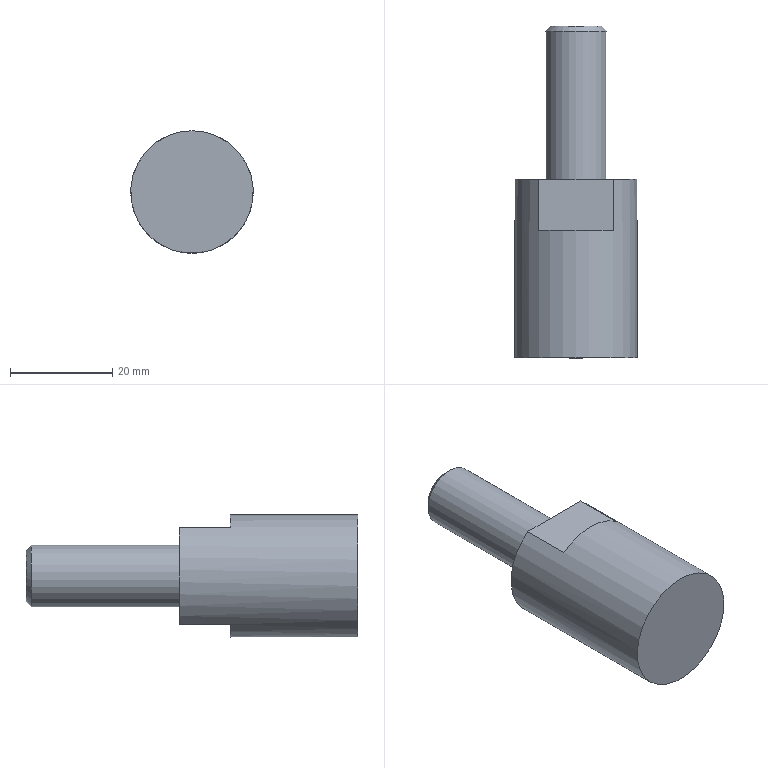Part | NX | features solid 2 | 1 solid | 10 faces | box 24 x 65 x 24 mm | volume 18709 mm3 | plane 7 | cylinder 2 | cone 1 | commonest cylinder face diameters 12 x1 24 x1
STEP:
#1=CARTESIAN_POINT('',(-265.,490.,-30.));
#2=VERTEX_POINT('',#1);
#3=CARTESIAN_POINT('',(-265.,490.,-25.));
#4=DIRECTION('',(0.,-1.,0.));
#5=DIRECTION('',(0.,0.,-1.));
#6=AXIS2_PLACEMENT_3D('',#3,#4,#5);
#7=CIRCLE('',#6,5.);
#8=EDGE_CURVE('',#2,#2,#7,.T.);
#9=ORIENTED_EDGE('',*,*,#8,.F.);
#10=EDGE_LOOP('',(#9));
#11=FACE_BOUND('',#10,.T.);
#12=CARTESIAN_POINT('',(-265.,490.,-25.));
#13=DIRECTION('',(0.,1.,0.));
#14=DIRECTION('',(0.,0.,-1.));
#15=AXIS2_PLACEMENT_3D('',#12,#13,#14);
#16=PLANE('',#15);
#17=ADVANCED_FACE('',(#11),#16,.T.);
#18=CARTESIAN_POINT('',(-265.,489.,-31.));
#19=VERTEX_POINT('',#18);
#20=CARTESIAN_POINT('',(-265.,489.,-25.));
#21=DIRECTION('',(0.,-1.,0.));
#22=DIRECTION('',(0.,0.,-1.));
#23=AXIS2_PLACEMENT_3D('',#20,#21,#22);
#24=CIRCLE('',#23,6.);
#25=EDGE_CURVE('',#19,#19,#24,.F.);
#26=ORIENTED_EDGE('',*,*,#25,.T.);
#27=EDGE_LOOP('',(#26));
#28=FACE_BOUND('',#27,.T.);
#29=ORIENTED_EDGE('',*,*,#8,.T.);
#30=EDGE_LOOP('',(#29));
#31=FACE_BOUND('',#30,.T.);
#32=CARTESIAN_POINT('',(-265.,490.,-25.));
#33=DIRECTION('',(0.,-1.,0.));
#34=DIRECTION('',(0.,0.,1.));
#35=AXIS2_PLACEMENT_3D('',#32,#33,#34);
#36=CONICAL_SURFACE('',#35,5.,0.7854);
#37=ADVANCED_FACE('',(#28,#31),#36,.T.);
#38=ORIENTED_EDGE('',*,*,#25,.F.);
#39=EDGE_LOOP('',(#38));
#40=FACE_BOUND('',#39,.T.);
#41=CARTESIAN_POINT('',(-265.,460.,-31.));
#42=VERTEX_POINT('',#41);
#43=CARTESIAN_POINT('',(-265.,460.,-25.));
#44=DIRECTION('',(0.,-1.,0.));
#45=DIRECTION('',(0.,0.,-1.));
#46=AXIS2_PLACEMENT_3D('',#43,#44,#45);
#47=CIRCLE('',#46,6.);
#48=EDGE_CURVE('',#42,#42,#47,.T.);
#49=ORIENTED_EDGE('',*,*,#48,.F.);
#50=EDGE_LOOP('',(#49));
#51=FACE_BOUND('',#50,.T.);
#52=CARTESIAN_POINT('',(-265.,460.,-25.));
#53=DIRECTION('',(0.,1.,0.));
#54=DIRECTION('',(0.,0.,-1.));
#55=AXIS2_PLACEMENT_3D('',#52,#53,#54);
#56=CYLINDRICAL_SURFACE('',#55,6.);
#57=ADVANCED_FACE('',(#40,#51),#56,.T.);
#58=CARTESIAN_POINT('',(-272.331,450.,-34.5));
#59=VERTEX_POINT('',#58);
#60=CARTESIAN_POINT('',(-257.669,450.,-34.5));
#61=VERTEX_POINT('',#60);
#62=CARTESIAN_POINT('',(-272.331,450.,-34.5));
#63=DIRECTION('',(1.,0.,0.));
#64=VECTOR('',#63,1000.);
#65=LINE('',#62,#64);
#66=EDGE_CURVE('',#59,#61,#65,.T.);
#67=ORIENTED_EDGE('',*,*,#66,.T.);
#68=CARTESIAN_POINT('',(-265.,450.,-25.));
#69=DIRECTION('',(0.,-1.,0.));
#70=DIRECTION('',(0.,0.,-1.));
#71=AXIS2_PLACEMENT_3D('',#68,#69,#70);
#72=CIRCLE('',#71,12.);
#73=EDGE_CURVE('',#59,#61,#72,.T.);
#74=ORIENTED_EDGE('',*,*,#73,.F.);
#75=EDGE_LOOP('',(#67,#74));
#76=FACE_BOUND('',#75,.T.);
#77=CARTESIAN_POINT('',(-272.331,450.,-25.));
#78=DIRECTION('',(0.,1.,0.));
#79=DIRECTION('',(0.,0.,-1.));
#80=AXIS2_PLACEMENT_3D('',#77,#78,#79);
#81=PLANE('',#80);
#82=ADVANCED_FACE('',(#76),#81,.T.);
#83=CARTESIAN_POINT('',(-257.669,450.,-15.5));
#84=VERTEX_POINT('',#83);
#85=CARTESIAN_POINT('',(-272.331,450.,-15.5));
#86=VERTEX_POINT('',#85);
#87=CARTESIAN_POINT('',(-265.,450.,-25.));
#88=DIRECTION('',(0.,-1.,0.));
#89=DIRECTION('',(0.,0.,-1.));
#90=AXIS2_PLACEMENT_3D('',#87,#88,#89);
#91=CIRCLE('',#90,12.);
#92=EDGE_CURVE('',#84,#86,#91,.T.);
#93=ORIENTED_EDGE('',*,*,#92,.F.);
#94=CARTESIAN_POINT('',(-272.331,450.,-15.5));
#95=DIRECTION('',(1.,0.,0.));
#96=VECTOR('',#95,1000.);
#97=LINE('',#94,#96);
#98=EDGE_CURVE('',#86,#84,#97,.T.);
#99=ORIENTED_EDGE('',*,*,#98,.F.);
#100=EDGE_LOOP('',(#93,#99));
#101=FACE_BOUND('',#100,.T.);
#102=CARTESIAN_POINT('',(-268.666,450.,-26.25));
#103=DIRECTION('',(0.,1.,0.));
#104=DIRECTION('',(0.,0.,-1.));
#105=AXIS2_PLACEMENT_3D('',#102,#103,#104);
#106=PLANE('',#105);
#107=ADVANCED_FACE('',(#101),#106,.T.);
#108=CARTESIAN_POINT('',(-272.331,460.,-15.5));
#109=VERTEX_POINT('',#108);
#110=CARTESIAN_POINT('',(-257.669,460.,-15.5));
#111=VERTEX_POINT('',#110);
#112=CARTESIAN_POINT('',(-272.331,460.,-15.5));
#113=DIRECTION('',(1.,0.,0.));
#114=VECTOR('',#113,1000.);
#115=LINE('',#112,#114);
#116=EDGE_CURVE('',#109,#111,#115,.T.);
#117=ORIENTED_EDGE('',*,*,#116,.F.);
#118=CARTESIAN_POINT('',(-272.331,450.,-15.5));
#119=DIRECTION('',(0.,1.,0.));
#120=VECTOR('',#119,1000.);
#121=LINE('',#118,#120);
#122=EDGE_CURVE('',#109,#86,#121,.F.);
#123=ORIENTED_EDGE('',*,*,#122,.T.);
#124=ORIENTED_EDGE('',*,*,#98,.T.);
#125=CARTESIAN_POINT('',(-257.669,450.,-15.5));
#126=DIRECTION('',(0.,1.,0.));
#127=VECTOR('',#126,1000.);
#128=LINE('',#125,#127);
#129=EDGE_CURVE('',#84,#111,#128,.T.);
#130=ORIENTED_EDGE('',*,*,#129,.T.);
#131=EDGE_LOOP('',(#117,#123,#124,#130));
#132=FACE_BOUND('',#131,.T.);
#133=CARTESIAN_POINT('',(-272.331,450.,-15.5));
#134=DIRECTION('',(0.,0.,-1.));
#135=DIRECTION('',(0.,-1.,0.));
#136=AXIS2_PLACEMENT_3D('',#133,#134,#135);
#137=PLANE('',#136);
#138=ADVANCED_FACE('',(#132),#137,.F.);
#139=ORIENTED_EDGE('',*,*,#48,.T.);
#140=EDGE_LOOP('',(#139));
#141=FACE_BOUND('',#140,.T.);
#142=CARTESIAN_POINT('',(-272.331,460.,-34.5));
#143=VERTEX_POINT('',#142);
#144=CARTESIAN_POINT('',(-265.,460.,-25.));
#145=DIRECTION('',(0.,-1.,0.));
#146=DIRECTION('',(0.,0.,-1.));
#147=AXIS2_PLACEMENT_3D('',#144,#145,#146);
#148=CIRCLE('',#147,12.);
#149=EDGE_CURVE('',#109,#143,#148,.T.);
#150=ORIENTED_EDGE('',*,*,#149,.F.);
#151=ORIENTED_EDGE('',*,*,#116,.T.);
#152=CARTESIAN_POINT('',(-257.669,460.,-34.5));
#153=VERTEX_POINT('',#152);
#154=CARTESIAN_POINT('',(-265.,460.,-25.));
#155=DIRECTION('',(0.,-1.,0.));
#156=DIRECTION('',(0.,0.,-1.));
#157=AXIS2_PLACEMENT_3D('',#154,#155,#156);
#158=CIRCLE('',#157,12.);
#159=EDGE_CURVE('',#153,#111,#158,.T.);
#160=ORIENTED_EDGE('',*,*,#159,.F.);
#161=CARTESIAN_POINT('',(-272.331,460.,-34.5));
#162=DIRECTION('',(1.,0.,0.));
#163=VECTOR('',#162,1000.);
#164=LINE('',#161,#163);
#165=EDGE_CURVE('',#143,#153,#164,.T.);
#166=ORIENTED_EDGE('',*,*,#165,.F.);
#167=EDGE_LOOP('',(#150,#151,#160,#166));
#168=FACE_BOUND('',#167,.T.);
#169=CARTESIAN_POINT('',(-265.,460.,-25.));
#170=DIRECTION('',(0.,1.,0.));
#171=DIRECTION('',(0.,0.,-1.));
#172=AXIS2_PLACEMENT_3D('',#169,#170,#171);
#173=PLANE('',#172);
#174=ADVANCED_FACE('',(#141,#168),#173,.T.);
#175=ORIENTED_EDGE('',*,*,#165,.T.);
#176=CARTESIAN_POINT('',(-257.669,450.,-34.5));
#177=DIRECTION('',(0.,1.,0.));
#178=VECTOR('',#177,1000.);
#179=LINE('',#176,#178);
#180=EDGE_CURVE('',#153,#61,#179,.F.);
#181=ORIENTED_EDGE('',*,*,#180,.T.);
#182=ORIENTED_EDGE('',*,*,#66,.F.);
#183=CARTESIAN_POINT('',(-272.331,450.,-34.5));
#184=DIRECTION('',(0.,1.,0.));
#185=VECTOR('',#184,1000.);
#186=LINE('',#183,#185);
#187=EDGE_CURVE('',#59,#143,#186,.T.);
#188=ORIENTED_EDGE('',*,*,#187,.T.);
#189=EDGE_LOOP('',(#175,#181,#182,#188));
#190=FACE_BOUND('',#189,.T.);
#191=CARTESIAN_POINT('',(-272.331,450.,-34.5));
#192=DIRECTION('',(0.,0.,-1.));
#193=DIRECTION('',(0.,-1.,0.));
#194=AXIS2_PLACEMENT_3D('',#191,#192,#193);
#195=PLANE('',#194);
#196=ADVANCED_FACE('',(#190),#195,.T.);
#197=CARTESIAN_POINT('',(-265.,425.,-13.));
#198=VERTEX_POINT('',#197);
#199=CARTESIAN_POINT('',(-265.,425.,-25.));
#200=DIRECTION('',(0.,-1.,0.));
#201=DIRECTION('',(0.,0.,1.));
#202=AXIS2_PLACEMENT_3D('',#199,#200,#201);
#203=CIRCLE('',#202,12.);
#204=EDGE_CURVE('',#198,#198,#203,.T.);
#205=ORIENTED_EDGE('',*,*,#204,.F.);
#206=EDGE_LOOP('',(#205));
#207=FACE_BOUND('',#206,.T.);
#208=ORIENTED_EDGE('',*,*,#187,.F.);
#209=ORIENTED_EDGE('',*,*,#73,.T.);
#210=ORIENTED_EDGE('',*,*,#180,.F.);
#211=ORIENTED_EDGE('',*,*,#159,.T.);
#212=ORIENTED_EDGE('',*,*,#129,.F.);
#213=ORIENTED_EDGE('',*,*,#92,.T.);
#214=ORIENTED_EDGE('',*,*,#122,.F.);
#215=ORIENTED_EDGE('',*,*,#149,.T.);
#216=EDGE_LOOP('',(#208,#209,#210,#211,#212,#213,#214,#215));
#217=FACE_BOUND('',#216,.T.);
#218=CARTESIAN_POINT('',(-265.,460.,-25.));
#219=DIRECTION('',(0.,-1.,0.));
#220=DIRECTION('',(0.,0.,1.));
#221=AXIS2_PLACEMENT_3D('',#218,#219,#220);
#222=CYLINDRICAL_SURFACE('',#221,12.);
#223=ADVANCED_FACE('',(#207,#217),#222,.T.);
#224=ORIENTED_EDGE('',*,*,#204,.T.);
#225=EDGE_LOOP('',(#224));
#226=FACE_BOUND('',#225,.T.);
#227=CARTESIAN_POINT('',(-77.42,425.,-459.905));
#228=DIRECTION('',(0.,1.,0.));
#229=DIRECTION('',(0.,0.,1.));
#230=AXIS2_PLACEMENT_3D('',#227,#228,#229);
#231=PLANE('',#230);
#232=ADVANCED_FACE('',(#226),#231,.F.);
#233=CLOSED_SHELL('',(#17,#37,#57,#82,#107,#138,#174,#196,#223,#232));
#234=MANIFOLD_SOLID_BREP('',#233);
#235=(LENGTH_UNIT()NAMED_UNIT(*)SI_UNIT(.MILLI.,.METRE.));
#236=UNCERTAINTY_MEASURE_WITH_UNIT(LENGTH_MEASURE(0.00001),#235,'','');
#237=(NAMED_UNIT(*)PLANE_ANGLE_UNIT()SI_UNIT($,.RADIAN.));
#238=(NAMED_UNIT(*)SI_UNIT($,.STERADIAN.)SOLID_ANGLE_UNIT());
#239=(GEOMETRIC_REPRESENTATION_CONTEXT(3)GLOBAL_UNCERTAINTY_ASSIGNED_CONTEXT((#236))GLOBAL_UNIT_ASSIGNED_CONTEXT((#235,#237,#238))REPRESENTATION_CONTEXT('',''));
#240=ADVANCED_BREP_SHAPE_REPRESENTATION('',(#234),#239);